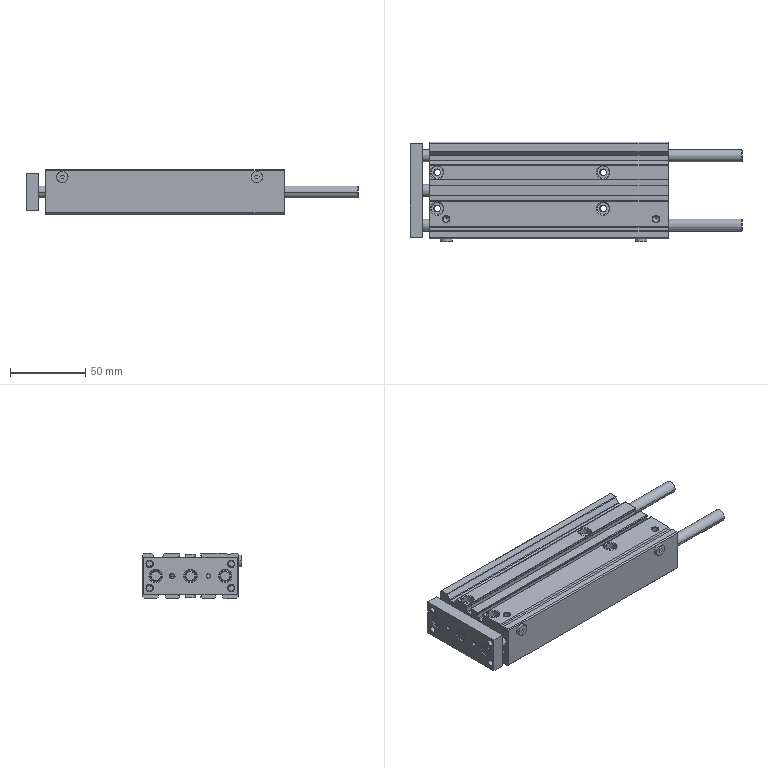Part | STEP file | 2 solids | 425 faces | box 220 x 66.1 x 30 mm | volume 246050 mm3 | cylinder 177 | plane 144 | cone 102 | torus 2 | commonest cylinder face diameters 8 x30 4.134 x28 3 x21 0.8 x20 0.4 x16 4.5 x8